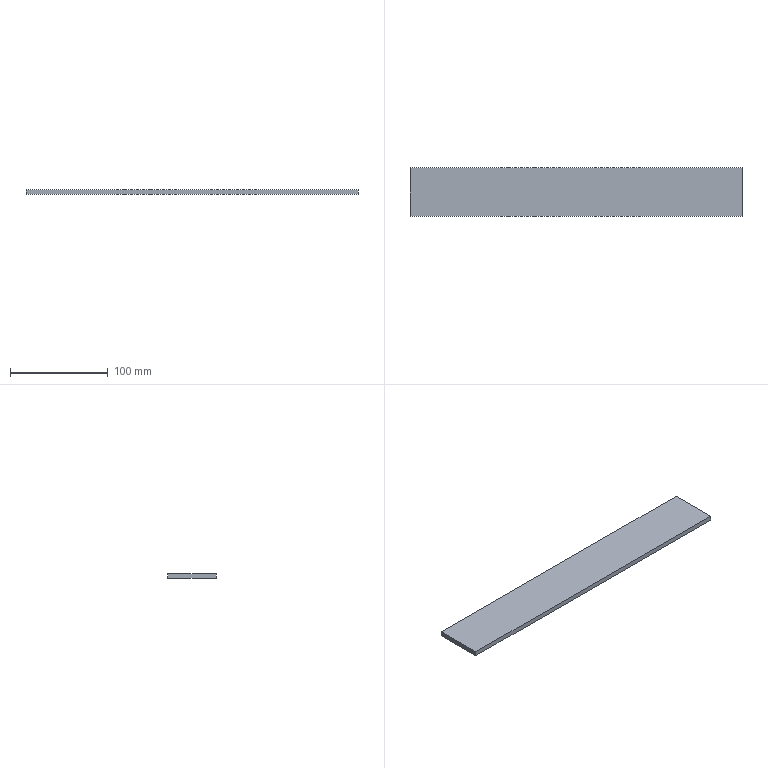Part | SolidWorks | features Extrusion 1 | 1 solid | 6 faces | box 340 x 50 x 5 mm | volume 85000 mm3 | plane 6
STEP:
#1=CARTESIAN_POINT('',(0.,50.,0.));
#2=VERTEX_POINT('',#1);
#3=CARTESIAN_POINT('',(0.,0.,0.));
#4=VERTEX_POINT('',#3);
#5=CARTESIAN_POINT('',(0.,50.,0.));
#6=DIRECTION('',(0.,-1.,0.));
#7=VECTOR('',#6,1000.);
#8=LINE('',#5,#7);
#9=EDGE_CURVE('',#2,#4,#8,.T.);
#10=ORIENTED_EDGE('',*,*,#9,.T.);
#11=CARTESIAN_POINT('',(0.,0.,5.));
#12=VERTEX_POINT('',#11);
#13=CARTESIAN_POINT('',(0.,0.,5.));
#14=DIRECTION('',(0.,0.,-1.));
#15=VECTOR('',#14,1000.);
#16=LINE('',#13,#15);
#17=EDGE_CURVE('',#12,#4,#16,.T.);
#18=ORIENTED_EDGE('',*,*,#17,.F.);
#19=CARTESIAN_POINT('',(0.,50.,5.));
#20=VERTEX_POINT('',#19);
#21=CARTESIAN_POINT('',(0.,50.,5.));
#22=DIRECTION('',(0.,-1.,0.));
#23=VECTOR('',#22,1000.);
#24=LINE('',#21,#23);
#25=EDGE_CURVE('',#20,#12,#24,.T.);
#26=ORIENTED_EDGE('',*,*,#25,.F.);
#27=CARTESIAN_POINT('',(0.,50.,5.));
#28=DIRECTION('',(0.,0.,-1.));
#29=VECTOR('',#28,1000.);
#30=LINE('',#27,#29);
#31=EDGE_CURVE('',#20,#2,#30,.T.);
#32=ORIENTED_EDGE('',*,*,#31,.T.);
#33=EDGE_LOOP('',(#10,#18,#26,#32));
#34=FACE_OUTER_BOUND('',#33,.T.);
#35=CARTESIAN_POINT('',(0.,50.,5.));
#36=DIRECTION('',(1.,0.,0.));
#37=DIRECTION('',(0.,0.,-1.));
#38=AXIS2_PLACEMENT_3D('',#35,#36,#37);
#39=PLANE('',#38);
#40=ADVANCED_FACE('',(#34),#39,.F.);
#41=CARTESIAN_POINT('',(340.,0.,0.));
#42=VERTEX_POINT('',#41);
#43=CARTESIAN_POINT('',(0.,0.,0.));
#44=DIRECTION('',(1.,0.,0.));
#45=VECTOR('',#44,1000.);
#46=LINE('',#43,#45);
#47=EDGE_CURVE('',#4,#42,#46,.T.);
#48=ORIENTED_EDGE('',*,*,#47,.T.);
#49=CARTESIAN_POINT('',(340.,0.,5.));
#50=VERTEX_POINT('',#49);
#51=CARTESIAN_POINT('',(340.,0.,5.));
#52=DIRECTION('',(0.,0.,-1.));
#53=VECTOR('',#52,1000.);
#54=LINE('',#51,#53);
#55=EDGE_CURVE('',#50,#42,#54,.T.);
#56=ORIENTED_EDGE('',*,*,#55,.F.);
#57=CARTESIAN_POINT('',(0.,0.,5.));
#58=DIRECTION('',(1.,0.,0.));
#59=VECTOR('',#58,1000.);
#60=LINE('',#57,#59);
#61=EDGE_CURVE('',#12,#50,#60,.T.);
#62=ORIENTED_EDGE('',*,*,#61,.F.);
#63=ORIENTED_EDGE('',*,*,#17,.T.);
#64=EDGE_LOOP('',(#48,#56,#62,#63));
#65=FACE_OUTER_BOUND('',#64,.T.);
#66=CARTESIAN_POINT('',(0.,0.,5.));
#67=DIRECTION('',(0.,1.,0.));
#68=DIRECTION('',(0.,0.,1.));
#69=AXIS2_PLACEMENT_3D('',#66,#67,#68);
#70=PLANE('',#69);
#71=ADVANCED_FACE('',(#65),#70,.F.);
#72=CARTESIAN_POINT('',(340.,50.,0.));
#73=VERTEX_POINT('',#72);
#74=CARTESIAN_POINT('',(340.,0.,0.));
#75=DIRECTION('',(0.,1.,0.));
#76=VECTOR('',#75,1000.);
#77=LINE('',#74,#76);
#78=EDGE_CURVE('',#42,#73,#77,.T.);
#79=ORIENTED_EDGE('',*,*,#78,.T.);
#80=CARTESIAN_POINT('',(340.,50.,5.));
#81=VERTEX_POINT('',#80);
#82=CARTESIAN_POINT('',(340.,50.,5.));
#83=DIRECTION('',(0.,0.,-1.));
#84=VECTOR('',#83,1000.);
#85=LINE('',#82,#84);
#86=EDGE_CURVE('',#81,#73,#85,.T.);
#87=ORIENTED_EDGE('',*,*,#86,.F.);
#88=CARTESIAN_POINT('',(340.,0.,5.));
#89=DIRECTION('',(0.,1.,0.));
#90=VECTOR('',#89,1000.);
#91=LINE('',#88,#90);
#92=EDGE_CURVE('',#50,#81,#91,.T.);
#93=ORIENTED_EDGE('',*,*,#92,.F.);
#94=ORIENTED_EDGE('',*,*,#55,.T.);
#95=EDGE_LOOP('',(#79,#87,#93,#94));
#96=FACE_OUTER_BOUND('',#95,.T.);
#97=CARTESIAN_POINT('',(340.,0.,5.));
#98=DIRECTION('',(-1.,0.,0.));
#99=DIRECTION('',(0.,0.,1.));
#100=AXIS2_PLACEMENT_3D('',#97,#98,#99);
#101=PLANE('',#100);
#102=ADVANCED_FACE('',(#96),#101,.F.);
#103=CARTESIAN_POINT('',(340.,50.,0.));
#104=DIRECTION('',(-1.,0.,0.));
#105=VECTOR('',#104,1000.);
#106=LINE('',#103,#105);
#107=EDGE_CURVE('',#73,#2,#106,.T.);
#108=ORIENTED_EDGE('',*,*,#107,.T.);
#109=ORIENTED_EDGE('',*,*,#31,.F.);
#110=CARTESIAN_POINT('',(340.,50.,5.));
#111=DIRECTION('',(-1.,0.,0.));
#112=VECTOR('',#111,1000.);
#113=LINE('',#110,#112);
#114=EDGE_CURVE('',#81,#20,#113,.T.);
#115=ORIENTED_EDGE('',*,*,#114,.F.);
#116=ORIENTED_EDGE('',*,*,#86,.T.);
#117=EDGE_LOOP('',(#108,#109,#115,#116));
#118=FACE_OUTER_BOUND('',#117,.T.);
#119=CARTESIAN_POINT('',(340.,50.,5.));
#120=DIRECTION('',(0.,-1.,0.));
#121=DIRECTION('',(0.,0.,-1.));
#122=AXIS2_PLACEMENT_3D('',#119,#120,#121);
#123=PLANE('',#122);
#124=ADVANCED_FACE('',(#118),#123,.F.);
#125=ORIENTED_EDGE('',*,*,#25,.T.);
#126=ORIENTED_EDGE('',*,*,#61,.T.);
#127=ORIENTED_EDGE('',*,*,#92,.T.);
#128=ORIENTED_EDGE('',*,*,#114,.T.);
#129=EDGE_LOOP('',(#125,#126,#127,#128));
#130=FACE_OUTER_BOUND('',#129,.T.);
#131=CARTESIAN_POINT('',(0.,0.,5.));
#132=DIRECTION('',(0.,0.,1.));
#133=DIRECTION('',(1.,0.,0.));
#134=AXIS2_PLACEMENT_3D('',#131,#132,#133);
#135=PLANE('',#134);
#136=ADVANCED_FACE('',(#130),#135,.T.);
#137=ORIENTED_EDGE('',*,*,#9,.F.);
#138=ORIENTED_EDGE('',*,*,#107,.F.);
#139=ORIENTED_EDGE('',*,*,#78,.F.);
#140=ORIENTED_EDGE('',*,*,#47,.F.);
#141=EDGE_LOOP('',(#137,#138,#139,#140));
#142=FACE_OUTER_BOUND('',#141,.T.);
#143=CARTESIAN_POINT('',(0.,0.,0.));
#144=DIRECTION('',(0.,0.,1.));
#145=DIRECTION('',(1.,0.,0.));
#146=AXIS2_PLACEMENT_3D('',#143,#144,#145);
#147=PLANE('',#146);
#148=ADVANCED_FACE('',(#142),#147,.F.);
#149=CLOSED_SHELL('',(#40,#71,#102,#124,#136,#148));
#150=MANIFOLD_SOLID_BREP('',#149);
#151=CARTESIAN_POINT('',(0.,0.,0.));
#152=DIRECTION('',(0.,0.,1.));
#153=DIRECTION('',(1.,0.,0.));
#154=AXIS2_PLACEMENT_3D('',#151,#152,#153);
#155=(LENGTH_UNIT()NAMED_UNIT(*)SI_UNIT(.MILLI.,.METRE.));
#156=UNCERTAINTY_MEASURE_WITH_UNIT(LENGTH_MEASURE(0.00001),#155,'','');
#157=(NAMED_UNIT(*)PLANE_ANGLE_UNIT()SI_UNIT($,.RADIAN.));
#158=(NAMED_UNIT(*)SI_UNIT($,.STERADIAN.)SOLID_ANGLE_UNIT());
#159=(GEOMETRIC_REPRESENTATION_CONTEXT(3)GLOBAL_UNCERTAINTY_ASSIGNED_CONTEXT((#156))GLOBAL_UNIT_ASSIGNED_CONTEXT((#155,#157,#158))REPRESENTATION_CONTEXT('',''));
#160=ADVANCED_BREP_SHAPE_REPRESENTATION('',(#150,#154),#159);